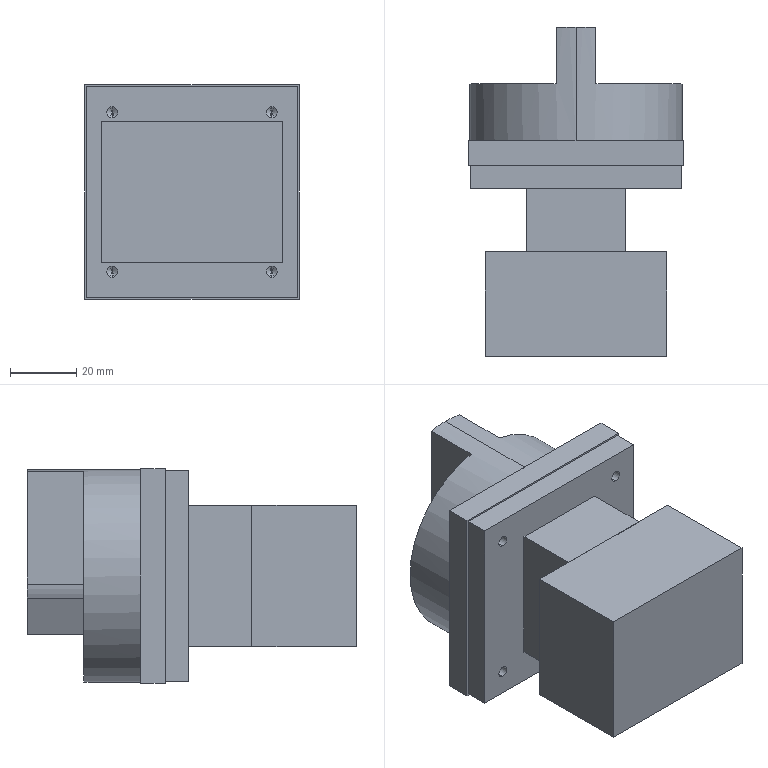Part | STEP file | power switch 2 | 5 solids | 61 faces | box 64.5 x 99 x 64.5 mm | volume 195044 mm3 | plane 32 | cylinder 21 | cone 8 | commonest cylinder face diameters 3.3 x16 20 x2 64 x2 53 x1